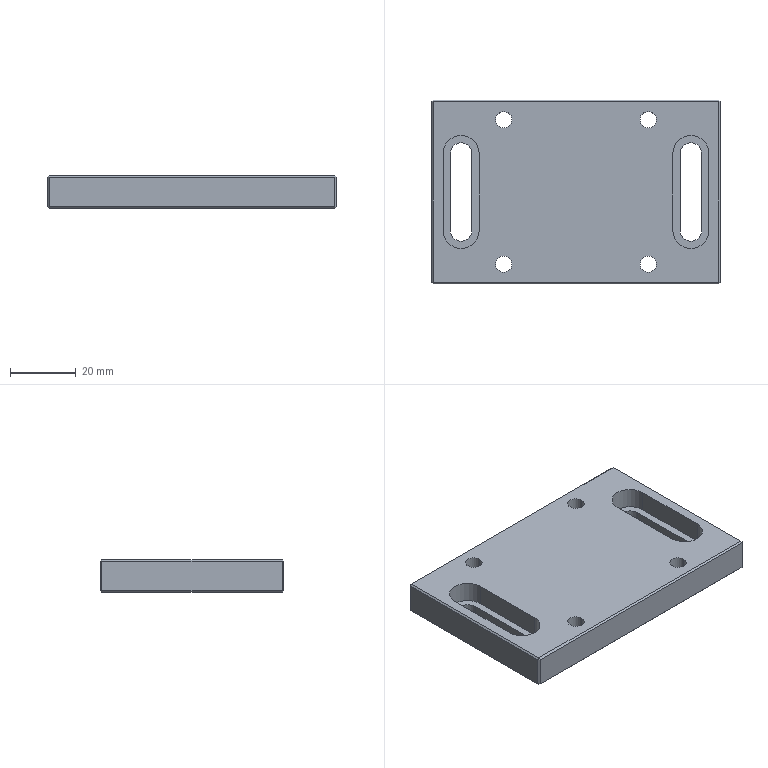Part | STEP file | 1 solid | 52 faces | box 88 x 56 x 10 mm | volume 42549 mm3 | plane 36 | cylinder 16 | commonest cylinder face diameters 5 x8 6.6 x4 11 x4